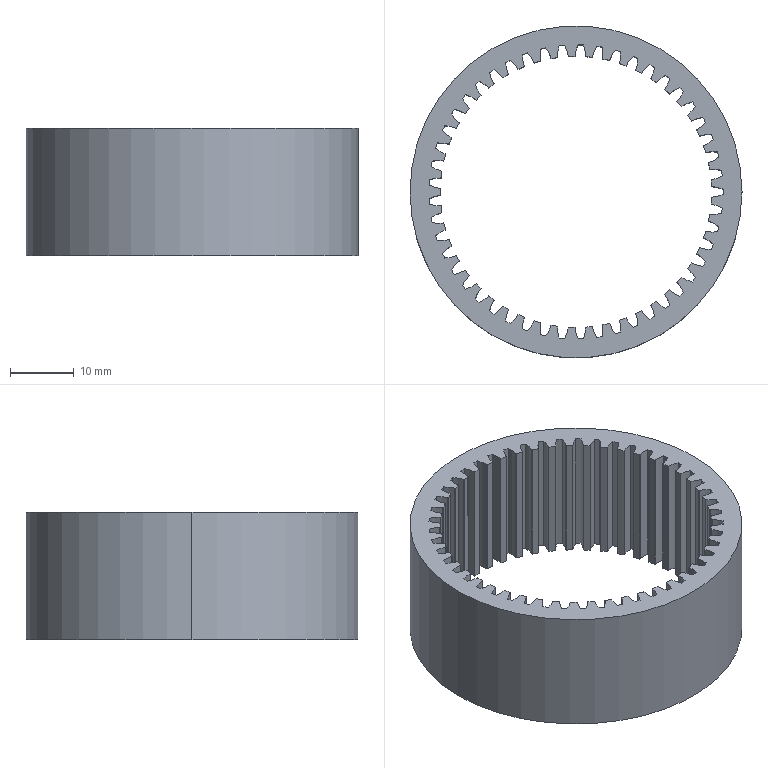Part | SolidWorks | features BaseBody 1 | 1 solid | 298 faces | box 52 x 52 x 20 mm | volume 11731 mm3 | plane 198 | spline 98 | cylinder 2 | commonest cylinder face diameters 52 x2